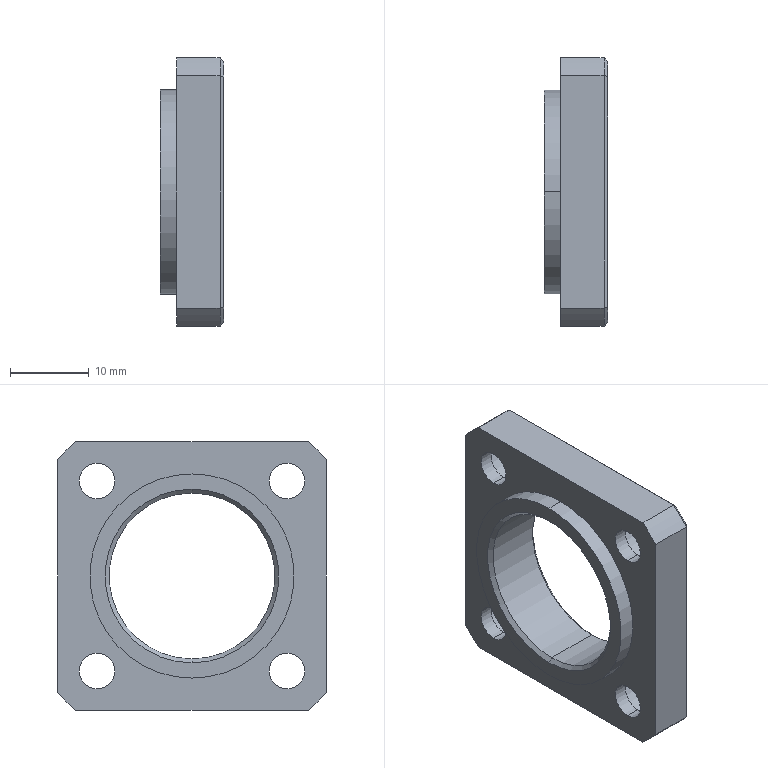Part | SolidWorks | features BaseBody 1 | 1 solid | 47 faces | box 8.1 x 34 x 34 mm | volume 4182 mm3 | cylinder 24 | plane 15 | cone 8 | commonest cylinder face diameters 4.5 x8 8 x8 45 x4 21 x2 25.85 x2
STEP:
#1=CARTESIAN_POINT('',(-6.,0.,12.925));
#2=VERTEX_POINT('',#1);
#3=CARTESIAN_POINT('',(-6.,0.,-12.925));
#4=VERTEX_POINT('',#3);
#5=CARTESIAN_POINT('',(-6.,0.,0.));
#6=DIRECTION('',(-1.,0.,0.));
#7=DIRECTION('',(0.,0.,1.));
#8=AXIS2_PLACEMENT_3D('',#5,#6,#7);
#9=CIRCLE('',#8,12.925);
#10=EDGE_CURVE('',#2,#4,#9,.T.);
#11=ORIENTED_EDGE('',*,*,#10,.T.);
#12=CARTESIAN_POINT('',(-8.1,0.,-12.925));
#13=VERTEX_POINT('',#12);
#14=CARTESIAN_POINT('',(0.,0.,-12.925));
#15=DIRECTION('',(-1.,0.,0.));
#16=VECTOR('',#15,1000.);
#17=LINE('',#14,#16);
#18=EDGE_CURVE('',#4,#13,#17,.T.);
#19=ORIENTED_EDGE('',*,*,#18,.T.);
#20=CARTESIAN_POINT('',(-8.1,0.,12.925));
#21=VERTEX_POINT('',#20);
#22=CARTESIAN_POINT('',(-8.1,0.,0.));
#23=DIRECTION('',(1.,0.,0.));
#24=DIRECTION('',(0.,0.,1.));
#25=AXIS2_PLACEMENT_3D('',#22,#23,#24);
#26=CIRCLE('',#25,12.925);
#27=EDGE_CURVE('',#13,#21,#26,.T.);
#28=ORIENTED_EDGE('',*,*,#27,.T.);
#29=CARTESIAN_POINT('',(0.,0.,12.925));
#30=DIRECTION('',(-1.,0.,0.));
#31=VECTOR('',#30,1000.);
#32=LINE('',#29,#31);
#33=EDGE_CURVE('',#2,#21,#32,.T.);
#34=ORIENTED_EDGE('',*,*,#33,.F.);
#35=EDGE_LOOP('',(#11,#19,#28,#34));
#36=FACE_OUTER_BOUND('',#35,.T.);
#37=CARTESIAN_POINT('',(0.,0.,0.));
#38=DIRECTION('',(-1.,0.,0.));
#39=DIRECTION('',(0.,0.,1.));
#40=AXIS2_PLACEMENT_3D('',#37,#38,#39);
#41=CYLINDRICAL_SURFACE('',#40,12.925);
#42=ADVANCED_FACE('',(#36),#41,.T.);
#43=CARTESIAN_POINT('',(-6.,12.021,-14.271));
#44=VERTEX_POINT('',#43);
#45=CARTESIAN_POINT('',(-6.,12.021,-9.771));
#46=VERTEX_POINT('',#45);
#47=CARTESIAN_POINT('',(-6.,12.021,-12.021));
#48=DIRECTION('',(-1.,0.,0.));
#49=DIRECTION('',(0.,0.,-1.));
#50=AXIS2_PLACEMENT_3D('',#47,#48,#49);
#51=CIRCLE('',#50,2.25);
#52=EDGE_CURVE('',#44,#46,#51,.T.);
#53=ORIENTED_EDGE('',*,*,#52,.T.);
#54=CARTESIAN_POINT('',(-4.2,12.021,-9.771));
#55=VERTEX_POINT('',#54);
#56=CARTESIAN_POINT('',(-8.1,12.021,-9.771));
#57=DIRECTION('',(1.,0.,0.));
#58=VECTOR('',#57,1000.);
#59=LINE('',#56,#58);
#60=EDGE_CURVE('',#46,#55,#59,.T.);
#61=ORIENTED_EDGE('',*,*,#60,.T.);
#62=CARTESIAN_POINT('',(-4.2,12.021,-14.271));
#63=VERTEX_POINT('',#62);
#64=CARTESIAN_POINT('',(-4.2,12.021,-12.021));
#65=DIRECTION('',(-1.,0.,0.));
#66=DIRECTION('',(0.,0.,-1.));
#67=AXIS2_PLACEMENT_3D('',#64,#65,#66);
#68=CIRCLE('',#67,2.25);
#69=EDGE_CURVE('',#63,#55,#68,.T.);
#70=ORIENTED_EDGE('',*,*,#69,.F.);
#71=CARTESIAN_POINT('',(-8.1,12.021,-14.271));
#72=DIRECTION('',(1.,0.,0.));
#73=VECTOR('',#72,1000.);
#74=LINE('',#71,#73);
#75=EDGE_CURVE('',#44,#63,#74,.T.);
#76=ORIENTED_EDGE('',*,*,#75,.F.);
#77=EDGE_LOOP('',(#53,#61,#70,#76));
#78=FACE_OUTER_BOUND('',#77,.T.);
#79=CARTESIAN_POINT('',(-8.1,12.021,-12.021));
#80=DIRECTION('',(1.,0.,0.));
#81=DIRECTION('',(0.,0.,-1.));
#82=AXIS2_PLACEMENT_3D('',#79,#80,#81);
#83=CYLINDRICAL_SURFACE('',#82,2.25);
#84=ADVANCED_FACE('',(#78),#83,.F.);
#85=CARTESIAN_POINT('',(-6.,-12.021,-14.271));
#86=VERTEX_POINT('',#85);
#87=CARTESIAN_POINT('',(-6.,-12.021,-9.771));
#88=VERTEX_POINT('',#87);
#89=CARTESIAN_POINT('',(-6.,-12.021,-12.021));
#90=DIRECTION('',(-1.,0.,0.));
#91=DIRECTION('',(0.,0.,-1.));
#92=AXIS2_PLACEMENT_3D('',#89,#90,#91);
#93=CIRCLE('',#92,2.25);
#94=EDGE_CURVE('',#86,#88,#93,.T.);
#95=ORIENTED_EDGE('',*,*,#94,.T.);
#96=CARTESIAN_POINT('',(-4.2,-12.021,-9.771));
#97=VERTEX_POINT('',#96);
#98=CARTESIAN_POINT('',(-8.1,-12.021,-9.771));
#99=DIRECTION('',(1.,0.,0.));
#100=VECTOR('',#99,1000.);
#101=LINE('',#98,#100);
#102=EDGE_CURVE('',#88,#97,#101,.T.);
#103=ORIENTED_EDGE('',*,*,#102,.T.);
#104=CARTESIAN_POINT('',(-4.2,-12.021,-14.271));
#105=VERTEX_POINT('',#104);
#106=CARTESIAN_POINT('',(-4.2,-12.021,-12.021));
#107=DIRECTION('',(-1.,0.,0.));
#108=DIRECTION('',(0.,0.,-1.));
#109=AXIS2_PLACEMENT_3D('',#106,#107,#108);
#110=CIRCLE('',#109,2.25);
#111=EDGE_CURVE('',#105,#97,#110,.T.);
#112=ORIENTED_EDGE('',*,*,#111,.F.);
#113=CARTESIAN_POINT('',(-8.1,-12.021,-14.271));
#114=DIRECTION('',(1.,0.,0.));
#115=VECTOR('',#114,1000.);
#116=LINE('',#113,#115);
#117=EDGE_CURVE('',#86,#105,#116,.T.);
#118=ORIENTED_EDGE('',*,*,#117,.F.);
#119=EDGE_LOOP('',(#95,#103,#112,#118));
#120=FACE_OUTER_BOUND('',#119,.T.);
#121=CARTESIAN_POINT('',(-8.1,-12.021,-12.021));
#122=DIRECTION('',(1.,0.,0.));
#123=DIRECTION('',(0.,0.,-1.));
#124=AXIS2_PLACEMENT_3D('',#121,#122,#123);
#125=CYLINDRICAL_SURFACE('',#124,2.25);
#126=ADVANCED_FACE('',(#120),#125,.F.);
#127=CARTESIAN_POINT('',(-6.,-12.021,9.771));
#128=VERTEX_POINT('',#127);
#129=CARTESIAN_POINT('',(-6.,-12.021,14.271));
#130=VERTEX_POINT('',#129);
#131=CARTESIAN_POINT('',(-6.,-12.021,12.021));
#132=DIRECTION('',(-1.,0.,0.));
#133=DIRECTION('',(0.,0.,-1.));
#134=AXIS2_PLACEMENT_3D('',#131,#132,#133);
#135=CIRCLE('',#134,2.25);
#136=EDGE_CURVE('',#128,#130,#135,.T.);
#137=ORIENTED_EDGE('',*,*,#136,.T.);
#138=CARTESIAN_POINT('',(-4.2,-12.021,14.271));
#139=VERTEX_POINT('',#138);
#140=CARTESIAN_POINT('',(-8.1,-12.021,14.271));
#141=DIRECTION('',(1.,0.,0.));
#142=VECTOR('',#141,1000.);
#143=LINE('',#140,#142);
#144=EDGE_CURVE('',#130,#139,#143,.T.);
#145=ORIENTED_EDGE('',*,*,#144,.T.);
#146=CARTESIAN_POINT('',(-4.2,-12.021,9.771));
#147=VERTEX_POINT('',#146);
#148=CARTESIAN_POINT('',(-4.2,-12.021,12.021));
#149=DIRECTION('',(-1.,0.,0.));
#150=DIRECTION('',(0.,0.,-1.));
#151=AXIS2_PLACEMENT_3D('',#148,#149,#150);
#152=CIRCLE('',#151,2.25);
#153=EDGE_CURVE('',#147,#139,#152,.T.);
#154=ORIENTED_EDGE('',*,*,#153,.F.);
#155=CARTESIAN_POINT('',(-8.1,-12.021,9.771));
#156=DIRECTION('',(1.,0.,0.));
#157=VECTOR('',#156,1000.);
#158=LINE('',#155,#157);
#159=EDGE_CURVE('',#128,#147,#158,.T.);
#160=ORIENTED_EDGE('',*,*,#159,.F.);
#161=EDGE_LOOP('',(#137,#145,#154,#160));
#162=FACE_OUTER_BOUND('',#161,.T.);
#163=CARTESIAN_POINT('',(-8.1,-12.021,12.021));
#164=DIRECTION('',(1.,0.,0.));
#165=DIRECTION('',(0.,0.,-1.));
#166=AXIS2_PLACEMENT_3D('',#163,#164,#165);
#167=CYLINDRICAL_SURFACE('',#166,2.25);
#168=ADVANCED_FACE('',(#162),#167,.F.);
#169=CARTESIAN_POINT('',(-6.,12.021,9.771));
#170=VERTEX_POINT('',#169);
#171=CARTESIAN_POINT('',(-6.,12.021,14.271));
#172=VERTEX_POINT('',#171);
#173=CARTESIAN_POINT('',(-6.,12.021,12.021));
#174=DIRECTION('',(-1.,0.,0.));
#175=DIRECTION('',(0.,0.,-1.));
#176=AXIS2_PLACEMENT_3D('',#173,#174,#175);
#177=CIRCLE('',#176,2.25);
#178=EDGE_CURVE('',#170,#172,#177,.T.);
#179=ORIENTED_EDGE('',*,*,#178,.T.);
#180=CARTESIAN_POINT('',(-4.2,12.021,14.271));
#181=VERTEX_POINT('',#180);
#182=CARTESIAN_POINT('',(-8.1,12.021,14.271));
#183=DIRECTION('',(1.,0.,0.));
#184=VECTOR('',#183,1000.);
#185=LINE('',#182,#184);
#186=EDGE_CURVE('',#172,#181,#185,.T.);
#187=ORIENTED_EDGE('',*,*,#186,.T.);
#188=CARTESIAN_POINT('',(-4.2,12.021,9.771));
#189=VERTEX_POINT('',#188);
#190=CARTESIAN_POINT('',(-4.2,12.021,12.021));
#191=DIRECTION('',(-1.,0.,0.));
#192=DIRECTION('',(0.,0.,-1.));
#193=AXIS2_PLACEMENT_3D('',#190,#191,#192);
#194=CIRCLE('',#193,2.25);
#195=EDGE_CURVE('',#189,#181,#194,.T.);
#196=ORIENTED_EDGE('',*,*,#195,.F.);
#197=CARTESIAN_POINT('',(-8.1,12.021,9.771));
#198=DIRECTION('',(1.,0.,0.));
#199=VECTOR('',#198,1000.);
#200=LINE('',#197,#199);
#201=EDGE_CURVE('',#170,#189,#200,.T.);
#202=ORIENTED_EDGE('',*,*,#201,.F.);
#203=EDGE_LOOP('',(#179,#187,#196,#202));
#204=FACE_OUTER_BOUND('',#203,.T.);
#205=CARTESIAN_POINT('',(-8.1,12.021,12.021));
#206=DIRECTION('',(1.,0.,0.));
#207=DIRECTION('',(0.,0.,-1.));
#208=AXIS2_PLACEMENT_3D('',#205,#206,#207);
#209=CYLINDRICAL_SURFACE('',#208,2.25);
#210=ADVANCED_FACE('',(#204),#209,.F.);
#211=CARTESIAN_POINT('',(-7.6,0.,-10.5));
#212=VERTEX_POINT('',#211);
#213=CARTESIAN_POINT('',(-7.6,0.,10.5));
#214=VERTEX_POINT('',#213);
#215=CARTESIAN_POINT('',(-7.6,0.,0.));
#216=DIRECTION('',(-1.,0.,0.));
#217=DIRECTION('',(0.,0.,1.));
#218=AXIS2_PLACEMENT_3D('',#215,#216,#217);
#219=CIRCLE('',#218,10.5);
#220=EDGE_CURVE('',#212,#214,#219,.T.);
#221=ORIENTED_EDGE('',*,*,#220,.F.);
#222=CARTESIAN_POINT('',(-8.1,0.,-11.));
#223=VERTEX_POINT('',#222);
#224=CARTESIAN_POINT('',(-8.1,0.,-11.));
#225=DIRECTION('',(-0.7071,0.,-0.7071));
#226=VECTOR('',#225,1000.);
#227=LINE('',#224,#226);
#228=EDGE_CURVE('',#212,#223,#227,.T.);
#229=ORIENTED_EDGE('',*,*,#228,.T.);
#230=CARTESIAN_POINT('',(-8.1,0.,11.));
#231=VERTEX_POINT('',#230);
#232=CARTESIAN_POINT('',(-8.1,0.,0.));
#233=DIRECTION('',(-1.,0.,0.));
#234=DIRECTION('',(0.,0.,1.));
#235=AXIS2_PLACEMENT_3D('',#232,#233,#234);
#236=CIRCLE('',#235,11.);
#237=EDGE_CURVE('',#223,#231,#236,.T.);
#238=ORIENTED_EDGE('',*,*,#237,.T.);
#239=CARTESIAN_POINT('',(-8.1,0.,11.));
#240=DIRECTION('',(-0.7071,0.,0.7071));
#241=VECTOR('',#240,1000.);
#242=LINE('',#239,#241);
#243=EDGE_CURVE('',#214,#231,#242,.T.);
#244=ORIENTED_EDGE('',*,*,#243,.F.);
#245=EDGE_LOOP('',(#221,#229,#238,#244));
#246=FACE_OUTER_BOUND('',#245,.T.);
#247=CARTESIAN_POINT('',(-8.1,0.,0.));
#248=DIRECTION('',(-1.,0.,0.));
#249=DIRECTION('',(0.,0.,1.));
#250=AXIS2_PLACEMENT_3D('',#247,#248,#249);
#251=CONICAL_SURFACE('',#250,11.,0.7854);
#252=ADVANCED_FACE('',(#246),#251,.F.);
#253=CARTESIAN_POINT('',(-4.2,12.021,-8.021));
#254=VERTEX_POINT('',#253);
#255=CARTESIAN_POINT('',(-4.2,12.021,-16.021));
#256=VERTEX_POINT('',#255);
#257=CARTESIAN_POINT('',(-4.2,12.021,-12.021));
#258=DIRECTION('',(1.,0.,0.));
#259=DIRECTION('',(0.,0.,-1.));
#260=AXIS2_PLACEMENT_3D('',#257,#258,#259);
#261=CIRCLE('',#260,4.);
#262=EDGE_CURVE('',#254,#256,#261,.T.);
#263=ORIENTED_EDGE('',*,*,#262,.F.);
#264=CARTESIAN_POINT('',(0.,12.021,-8.021));
#265=VERTEX_POINT('',#264);
#266=CARTESIAN_POINT('',(-8.1,12.021,-8.021));
#267=DIRECTION('',(1.,0.,0.));
#268=VECTOR('',#267,1000.);
#269=LINE('',#266,#268);
#270=EDGE_CURVE('',#254,#265,#269,.T.);
#271=ORIENTED_EDGE('',*,*,#270,.T.);
#272=CARTESIAN_POINT('',(0.,12.021,-16.021));
#273=VERTEX_POINT('',#272);
#274=CARTESIAN_POINT('',(0.,12.021,-12.021));
#275=DIRECTION('',(-1.,0.,0.));
#276=DIRECTION('',(0.,0.,-1.));
#277=AXIS2_PLACEMENT_3D('',#274,#275,#276);
#278=CIRCLE('',#277,4.);
#279=EDGE_CURVE('',#273,#265,#278,.T.);
#280=ORIENTED_EDGE('',*,*,#279,.F.);
#281=CARTESIAN_POINT('',(-8.1,12.021,-16.021));
#282=DIRECTION('',(1.,0.,0.));
#283=VECTOR('',#282,1000.);
#284=LINE('',#281,#283);
#285=EDGE_CURVE('',#256,#273,#284,.T.);
#286=ORIENTED_EDGE('',*,*,#285,.F.);
#287=EDGE_LOOP('',(#263,#271,#280,#286));
#288=FACE_OUTER_BOUND('',#287,.T.);
#289=CARTESIAN_POINT('',(-8.1,12.021,-12.021));
#290=DIRECTION('',(1.,0.,0.));
#291=DIRECTION('',(0.,0.,-1.));
#292=AXIS2_PLACEMENT_3D('',#289,#290,#291);
#293=CYLINDRICAL_SURFACE('',#292,4.);
#294=ADVANCED_FACE('',(#288),#293,.F.);
#295=CARTESIAN_POINT('',(-4.2,-12.021,-8.021));
#296=VERTEX_POINT('',#295);
#297=CARTESIAN_POINT('',(-4.2,-12.021,-16.021));
#298=VERTEX_POINT('',#297);
#299=CARTESIAN_POINT('',(-4.2,-12.021,-12.021));
#300=DIRECTION('',(1.,0.,0.));
#301=DIRECTION('',(0.,0.,-1.));
#302=AXIS2_PLACEMENT_3D('',#299,#300,#301);
#303=CIRCLE('',#302,4.);
#304=EDGE_CURVE('',#296,#298,#303,.T.);
#305=ORIENTED_EDGE('',*,*,#304,.F.);
#306=CARTESIAN_POINT('',(0.,-12.021,-8.021));
#307=VERTEX_POINT('',#306);
#308=CARTESIAN_POINT('',(-8.1,-12.021,-8.021));
#309=DIRECTION('',(1.,0.,0.));
#310=VECTOR('',#309,1000.);
#311=LINE('',#308,#310);
#312=EDGE_CURVE('',#296,#307,#311,.T.);
#313=ORIENTED_EDGE('',*,*,#312,.T.);
#314=CARTESIAN_POINT('',(0.,-12.021,-16.021));
#315=VERTEX_POINT('',#314);
#316=CARTESIAN_POINT('',(0.,-12.021,-12.021));
#317=DIRECTION('',(-1.,0.,0.));
#318=DIRECTION('',(0.,0.,-1.));
#319=AXIS2_PLACEMENT_3D('',#316,#317,#318);
#320=CIRCLE('',#319,4.);
#321=EDGE_CURVE('',#315,#307,#320,.T.);
#322=ORIENTED_EDGE('',*,*,#321,.F.);
#323=CARTESIAN_POINT('',(-8.1,-12.021,-16.021));
#324=DIRECTION('',(1.,0.,0.));
#325=VECTOR('',#324,1000.);
#326=LINE('',#323,#325);
#327=EDGE_CURVE('',#298,#315,#326,.T.);
#328=ORIENTED_EDGE('',*,*,#327,.F.);
#329=EDGE_LOOP('',(#305,#313,#322,#328));
#330=FACE_OUTER_BOUND('',#329,.T.);
#331=CARTESIAN_POINT('',(-8.1,-12.021,-12.021));
#332=DIRECTION('',(1.,0.,0.));
#333=DIRECTION('',(0.,0.,-1.));
#334=AXIS2_PLACEMENT_3D('',#331,#332,#333);
#335=CYLINDRICAL_SURFACE('',#334,4.);
#336=ADVANCED_FACE('',(#330),#335,.F.);
#337=CARTESIAN_POINT('',(-4.2,-12.021,16.021));
#338=VERTEX_POINT('',#337);
#339=CARTESIAN_POINT('',(-4.2,-12.021,8.021));
#340=VERTEX_POINT('',#339);
#341=CARTESIAN_POINT('',(-4.2,-12.021,12.021));
#342=DIRECTION('',(1.,0.,0.));
#343=DIRECTION('',(0.,0.,-1.));
#344=AXIS2_PLACEMENT_3D('',#341,#342,#343);
#345=CIRCLE('',#344,4.);
#346=EDGE_CURVE('',#338,#340,#345,.T.);
#347=ORIENTED_EDGE('',*,*,#346,.F.);
#348=CARTESIAN_POINT('',(0.,-12.021,16.021));
#349=VERTEX_POINT('',#348);
#350=CARTESIAN_POINT('',(-8.1,-12.021,16.021));
#351=DIRECTION('',(1.,0.,0.));
#352=VECTOR('',#351,1000.);
#353=LINE('',#350,#352);
#354=EDGE_CURVE('',#338,#349,#353,.T.);
#355=ORIENTED_EDGE('',*,*,#354,.T.);
#356=CARTESIAN_POINT('',(0.,-12.021,8.021));
#357=VERTEX_POINT('',#356);
#358=CARTESIAN_POINT('',(0.,-12.021,12.021));
#359=DIRECTION('',(-1.,0.,0.));
#360=DIRECTION('',(0.,0.,-1.));
#361=AXIS2_PLACEMENT_3D('',#358,#359,#360);
#362=CIRCLE('',#361,4.);
#363=EDGE_CURVE('',#357,#349,#362,.T.);
#364=ORIENTED_EDGE('',*,*,#363,.F.);
#365=CARTESIAN_POINT('',(-8.1,-12.021,8.021));
#366=DIRECTION('',(1.,0.,0.));
#367=VECTOR('',#366,1000.);
#368=LINE('',#365,#367);
#369=EDGE_CURVE('',#340,#357,#368,.T.);
#370=ORIENTED_EDGE('',*,*,#369,.F.);
#371=EDGE_LOOP('',(#347,#355,#364,#370));
#372=FACE_OUTER_BOUND('',#371,.T.);
#373=CARTESIAN_POINT('',(-8.1,-12.021,12.021));
#374=DIRECTION('',(1.,0.,0.));
#375=DIRECTION('',(0.,0.,-1.));
#376=AXIS2_PLACEMENT_3D('',#373,#374,#375);
#377=CYLINDRICAL_SURFACE('',#376,4.);
#378=ADVANCED_FACE('',(#372),#377,.F.);
#379=CARTESIAN_POINT('',(-4.2,12.021,16.021));
#380=VERTEX_POINT('',#379);
#381=CARTESIAN_POINT('',(-4.2,12.021,8.021));
#382=VERTEX_POINT('',#381);
#383=CARTESIAN_POINT('',(-4.2,12.021,12.021));
#384=DIRECTION('',(1.,0.,0.));
#385=DIRECTION('',(0.,0.,-1.));
#386=AXIS2_PLACEMENT_3D('',#383,#384,#385);
#387=CIRCLE('',#386,4.);
#388=EDGE_CURVE('',#380,#382,#387,.T.);
#389=ORIENTED_EDGE('',*,*,#388,.F.);
#390=CARTESIAN_POINT('',(0.,12.021,16.021));
#391=VERTEX_POINT('',#390);
#392=CARTESIAN_POINT('',(-8.1,12.021,16.021));
#393=DIRECTION('',(1.,0.,0.));
#394=VECTOR('',#393,1000.);
#395=LINE('',#392,#394);
#396=EDGE_CURVE('',#380,#391,#395,.T.);
#397=ORIENTED_EDGE('',*,*,#396,.T.);
#398=CARTESIAN_POINT('',(0.,12.021,8.021));
#399=VERTEX_POINT('',#398);
#400=CARTESIAN_POINT('',(0.,12.021,12.021));
#401=DIRECTION('',(-1.,0.,0.));
#402=DIRECTION('',(0.,0.,-1.));
#403=AXIS2_PLACEMENT_3D('',#400,#401,#402);
#404=CIRCLE('',#403,4.);
#405=EDGE_CURVE('',#399,#391,#404,.T.);
#406=ORIENTED_EDGE('',*,*,#405,.F.);
#407=CARTESIAN_POINT('',(-8.1,12.021,8.021));
#408=DIRECTION('',(1.,0.,0.));
#409=VECTOR('',#408,1000.);
#410=LINE('',#407,#409);
#411=EDGE_CURVE('',#382,#399,#410,.T.);
#412=ORIENTED_EDGE('',*,*,#411,.F.);
#413=EDGE_LOOP('',(#389,#397,#406,#412));
#414=FACE_OUTER_BOUND('',#413,.T.);
#415=CARTESIAN_POINT('',(-8.1,12.021,12.021));
#416=DIRECTION('',(1.,0.,0.));
#417=DIRECTION('',(0.,0.,-1.));
#418=AXIS2_PLACEMENT_3D('',#415,#416,#417);
#419=CYLINDRICAL_SURFACE('',#418,4.);
#420=ADVANCED_FACE('',(#414),#419,.F.);
#421=CARTESIAN_POINT('',(-0.5,0.,-10.5));
#422=VERTEX_POINT('',#421);
#423=CARTESIAN_POINT('',(-0.5,0.,10.5));
#424=VERTEX_POINT('',#423);
#425=CARTESIAN_POINT('',(-0.5,0.,0.));
#426=DIRECTION('',(-1.,0.,0.));
#427=DIRECTION('',(0.,0.,1.));
#428=AXIS2_PLACEMENT_3D('',#425,#426,#427);
#429=CIRCLE('',#428,10.5);
#430=EDGE_CURVE('',#422,#424,#429,.T.);
#431=ORIENTED_EDGE('',*,*,#430,.F.);
#432=CARTESIAN_POINT('',(0.,0.,-10.5));
#433=DIRECTION('',(-1.,0.,0.));
#434=VECTOR('',#433,1000.);
#435=LINE('',#432,#434);
#436=EDGE_CURVE('',#422,#212,#435,.T.);
#437=ORIENTED_EDGE('',*,*,#436,.T.);
#438=ORIENTED_EDGE('',*,*,#220,.T.);
#439=CARTESIAN_POINT('',(0.,0.,10.5));
#440=DIRECTION('',(-1.,0.,0.));
#441=VECTOR('',#440,1000.);
#442=LINE('',#439,#441);
#443=EDGE_CURVE('',#424,#214,#442,.T.);
#444=ORIENTED_EDGE('',*,*,#443,.F.);
#445=EDGE_LOOP('',(#431,#437,#438,#444));
#446=FACE_OUTER_BOUND('',#445,.T.);
#447=CARTESIAN_POINT('',(0.,0.,0.));
#448=DIRECTION('',(-1.,0.,0.));
#449=DIRECTION('',(0.,0.,1.));
#450=AXIS2_PLACEMENT_3D('',#447,#448,#449);
#451=CYLINDRICAL_SURFACE('',#450,10.5);
#452=ADVANCED_FACE('',(#446),#451,.F.);
#453=ORIENTED_EDGE('',*,*,#430,.T.);
#454=CARTESIAN_POINT('',(0.,0.,11.));
#455=VERTEX_POINT('',#454);
#456=CARTESIAN_POINT('',(0.,0.,11.));
#457=DIRECTION('',(0.7071,0.,0.7071));
#458=VECTOR('',#457,1000.);
#459=LINE('',#456,#458);
#460=EDGE_CURVE('',#424,#455,#459,.T.);
#461=ORIENTED_EDGE('',*,*,#460,.T.);
#462=CARTESIAN_POINT('',(0.,0.,-11.));
#463=VERTEX_POINT('',#462);
#464=CARTESIAN_POINT('',(0.,0.,0.));
#465=DIRECTION('',(1.,0.,0.));
#466=DIRECTION('',(0.,0.,-1.));
#467=AXIS2_PLACEMENT_3D('',#464,#465,#466);
#468=CIRCLE('',#467,11.);
#469=EDGE_CURVE('',#455,#463,#468,.T.);
#470=ORIENTED_EDGE('',*,*,#469,.T.);
#471=CARTESIAN_POINT('',(0.,0.,-11.));
#472=DIRECTION('',(0.7071,0.,-0.7071));
#473=VECTOR('',#472,1000.);
#474=LINE('',#471,#473);
#475=EDGE_CURVE('',#422,#463,#474,.T.);
#476=ORIENTED_EDGE('',*,*,#475,.F.);
#477=EDGE_LOOP('',(#453,#461,#470,#476));
#478=FACE_OUTER_BOUND('',#477,.T.);
#479=CARTESIAN_POINT('',(0.,0.,0.));
#480=DIRECTION('',(1.,0.,0.));
#481=DIRECTION('',(0.,0.,-1.));
#482=AXIS2_PLACEMENT_3D('',#479,#480,#481);
#483=CONICAL_SURFACE('',#482,11.,0.7854);
#484=ADVANCED_FACE('',(#478),#483,.F.);
#485=ORIENTED_EDGE('',*,*,#10,.F.);
#486=CARTESIAN_POINT('',(-6.,0.,0.));
#487=DIRECTION('',(-1.,0.,0.));
#488=DIRECTION('',(0.,0.,1.));
#489=AXIS2_PLACEMENT_3D('',#486,#487,#488);
#490=CIRCLE('',#489,12.925);
#491=EDGE_CURVE('',#4,#2,#490,.T.);
#492=ORIENTED_EDGE('',*,*,#491,.F.);
#493=EDGE_LOOP('',(#485,#492));
#494=FACE_BOUND('',#493,.T.);
#495=ORIENTED_EDGE('',*,*,#52,.F.);
#496=CARTESIAN_POINT('',(-6.,12.021,-12.021));
#497=DIRECTION('',(-1.,0.,0.));
#498=DIRECTION('',(0.,0.,-1.));
#499=AXIS2_PLACEMENT_3D('',#496,#497,#498);
#500=CIRCLE('',#499,2.25);
#501=EDGE_CURVE('',#46,#44,#500,.T.);
#502=ORIENTED_EDGE('',*,*,#501,.F.);
#503=EDGE_LOOP('',(#495,#502));
#504=FACE_BOUND('',#503,.T.);
#505=ORIENTED_EDGE('',*,*,#94,.F.);
#506=CARTESIAN_POINT('',(-6.,-12.021,-12.021));
#507=DIRECTION('',(-1.,0.,0.));
#508=DIRECTION('',(0.,0.,-1.));
#509=AXIS2_PLACEMENT_3D('',#506,#507,#508);
#510=CIRCLE('',#509,2.25);
#511=EDGE_CURVE('',#88,#86,#510,.T.);
#512=ORIENTED_EDGE('',*,*,#511,.F.);
#513=EDGE_LOOP('',(#505,#512));
#514=FACE_BOUND('',#513,.T.);
#515=ORIENTED_EDGE('',*,*,#136,.F.);
#516=CARTESIAN_POINT('',(-6.,-12.021,12.021));
#517=DIRECTION('',(-1.,0.,0.));
#518=DIRECTION('',(0.,0.,-1.));
#519=AXIS2_PLACEMENT_3D('',#516,#517,#518);
#520=CIRCLE('',#519,2.25);
#521=EDGE_CURVE('',#130,#128,#520,.T.);
#522=ORIENTED_EDGE('',*,*,#521,.F.);
#523=EDGE_LOOP('',(#515,#522));
#524=FACE_BOUND('',#523,.T.);
#525=ORIENTED_EDGE('',*,*,#178,.F.);
#526=CARTESIAN_POINT('',(-6.,12.021,12.021));
#527=DIRECTION('',(-1.,0.,0.));
#528=DIRECTION('',(0.,0.,-1.));
#529=AXIS2_PLACEMENT_3D('',#526,#527,#528);
#530=CIRCLE('',#529,2.25);
#531=EDGE_CURVE('',#172,#170,#530,.T.);
#532=ORIENTED_EDGE('',*,*,#531,.F.);
#533=EDGE_LOOP('',(#525,#532));
#534=FACE_BOUND('',#533,.T.);
#535=CARTESIAN_POINT('',(-6.,14.739,-17.));
#536=VERTEX_POINT('',#535);
#537=CARTESIAN_POINT('',(-6.,17.,-14.739));
#538=VERTEX_POINT('',#537);
#539=CARTESIAN_POINT('',(-6.,0.,0.));
#540=DIRECTION('',(1.,0.,0.));
#541=DIRECTION('',(0.,0.,1.));
#542=AXIS2_PLACEMENT_3D('',#539,#540,#541);
#543=CIRCLE('',#542,22.5);
#544=EDGE_CURVE('',#536,#538,#543,.T.);
#545=ORIENTED_EDGE('',*,*,#544,.F.);
#546=CARTESIAN_POINT('',(-6.,-14.739,-17.));
#547=VERTEX_POINT('',#546);
#548=CARTESIAN_POINT('',(-6.,12.925,-17.));
#549=DIRECTION('',(0.,1.,0.));
#550=VECTOR('',#549,1000.);
#551=LINE('',#548,#550);
#552=EDGE_CURVE('',#547,#536,#551,.T.);
#553=ORIENTED_EDGE('',*,*,#552,.F.);
#554=CARTESIAN_POINT('',(-6.,-17.,-14.739));
#555=VERTEX_POINT('',#554);
#556=CARTESIAN_POINT('',(-6.,0.,0.));
#557=DIRECTION('',(1.,0.,0.));
#558=DIRECTION('',(0.,0.,1.));
#559=AXIS2_PLACEMENT_3D('',#556,#557,#558);
#560=CIRCLE('',#559,22.5);
#561=EDGE_CURVE('',#555,#547,#560,.T.);
#562=ORIENTED_EDGE('',*,*,#561,.F.);
#563=CARTESIAN_POINT('',(-6.,-17.,14.739));
#564=VERTEX_POINT('',#563);
#565=CARTESIAN_POINT('',(-6.,-17.,0.));
#566=DIRECTION('',(0.,0.,-1.));
#567=VECTOR('',#566,1000.);
#568=LINE('',#565,#567);
#569=EDGE_CURVE('',#564,#555,#568,.T.);
#570=ORIENTED_EDGE('',*,*,#569,.F.);
#571=CARTESIAN_POINT('',(-6.,-14.739,17.));
#572=VERTEX_POINT('',#571);
#573=CARTESIAN_POINT('',(-6.,0.,0.));
#574=DIRECTION('',(1.,0.,0.));
#575=DIRECTION('',(0.,0.,1.));
#576=AXIS2_PLACEMENT_3D('',#573,#574,#575);
#577=CIRCLE('',#576,22.5);
#578=EDGE_CURVE('',#572,#564,#577,.T.);
#579=ORIENTED_EDGE('',*,*,#578,.F.);
#580=CARTESIAN_POINT('',(-6.,14.739,17.));
#581=VERTEX_POINT('',#580);
#582=CARTESIAN_POINT('',(-6.,12.925,17.));
#583=DIRECTION('',(0.,-1.,0.));
#584=VECTOR('',#583,1000.);
#585=LINE('',#582,#584);
#586=EDGE_CURVE('',#581,#572,#585,.T.);
#587=ORIENTED_EDGE('',*,*,#586,.F.);
#588=CARTESIAN_POINT('',(-6.,17.,14.739));
#589=VERTEX_POINT('',#588);
#590=CARTESIAN_POINT('',(-6.,0.,0.));
#591=DIRECTION('',(1.,0.,0.));
#592=DIRECTION('',(0.,0.,1.));
#593=AXIS2_PLACEMENT_3D('',#590,#591,#592);
#594=CIRCLE('',#593,22.5);
#595=EDGE_CURVE('',#589,#581,#594,.T.);
#596=ORIENTED_EDGE('',*,*,#595,.F.);
#597=CARTESIAN_POINT('',(-6.,17.,0.));
#598=DIRECTION('',(0.,0.,1.));
#599=VECTOR('',#598,1000.);
#600=LINE('',#597,#599);
#601=EDGE_CURVE('',#538,#589,#600,.T.);
#602=ORIENTED_EDGE('',*,*,#601,.F.);
#603=EDGE_LOOP('',(#545,#553,#562,#570,#579,#587,#596,#602));
#604=FACE_OUTER_BOUND('',#603,.T.);
#605=CARTESIAN_POINT('',(-6.,12.925,0.));
#606=DIRECTION('',(1.,0.,0.));
#607=DIRECTION('',(0.,0.,-1.));
#608=AXIS2_PLACEMENT_3D('',#605,#606,#607);
#609=PLANE('',#608);
#610=ADVANCED_FACE('',(#494,#504,#514,#524,#534,#604),#609,.F.);
#611=ORIENTED_EDGE('',*,*,#18,.F.);
#612=ORIENTED_EDGE('',*,*,#491,.T.);
#613=ORIENTED_EDGE('',*,*,#33,.T.);
#614=CARTESIAN_POINT('',(-8.1,0.,0.));
#615=DIRECTION('',(1.,0.,0.));
#616=DIRECTION('',(0.,0.,1.));
#617=AXIS2_PLACEMENT_3D('',#614,#615,#616);
#618=CIRCLE('',#617,12.925);
#619=EDGE_CURVE('',#21,#13,#618,.T.);
#620=ORIENTED_EDGE('',*,*,#619,.T.);
#621=EDGE_LOOP('',(#611,#612,#613,#620));
#622=FACE_OUTER_BOUND('',#621,.T.);
#623=CARTESIAN_POINT('',(0.,0.,0.));
#624=DIRECTION('',(-1.,0.,0.));
#625=DIRECTION('',(0.,0.,1.));
#626=AXIS2_PLACEMENT_3D('',#623,#624,#625);
#627=CYLINDRICAL_SURFACE('',#626,12.925);
#628=ADVANCED_FACE('',(#622),#627,.T.);
#629=ORIENTED_EDGE('',*,*,#60,.F.);
#630=ORIENTED_EDGE('',*,*,#501,.T.);
#631=ORIENTED_EDGE('',*,*,#75,.T.);
#632=CARTESIAN_POINT('',(-4.2,12.021,-12.021));
#633=DIRECTION('',(-1.,0.,0.));
#634=DIRECTION('',(0.,0.,-1.));
#635=AXIS2_PLACEMENT_3D('',#632,#633,#634);
#636=CIRCLE('',#635,2.25);
#637=EDGE_CURVE('',#55,#63,#636,.T.);
#638=ORIENTED_EDGE('',*,*,#637,.F.);
#639=EDGE_LOOP('',(#629,#630,#631,#638));
#640=FACE_OUTER_BOUND('',#639,.T.);
#641=CARTESIAN_POINT('',(-8.1,12.021,-12.021));
#642=DIRECTION('',(1.,0.,0.));
#643=DIRECTION('',(0.,0.,-1.));
#644=AXIS2_PLACEMENT_3D('',#641,#642,#643);
#645=CYLINDRICAL_SURFACE('',#644,2.25);
#646=ADVANCED_FACE('',(#640),#645,.F.);
#647=ORIENTED_EDGE('',*,*,#102,.F.);
#648=ORIENTED_EDGE('',*,*,#511,.T.);
#649=ORIENTED_EDGE('',*,*,#117,.T.);
#650=CARTESIAN_POINT('',(-4.2,-12.021,-12.021));
#651=DIRECTION('',(-1.,0.,0.));
#652=DIRECTION('',(0.,0.,-1.));
#653=AXIS2_PLACEMENT_3D('',#650,#651,#652);
#654=CIRCLE('',#653,2.25);
#655=EDGE_CURVE('',#97,#105,#654,.T.);
#656=ORIENTED_EDGE('',*,*,#655,.F.);
#657=EDGE_LOOP('',(#647,#648,#649,#656));
#658=FACE_OUTER_BOUND('',#657,.T.);
#659=CARTESIAN_POINT('',(-8.1,-12.021,-12.021));
#660=DIRECTION('',(1.,0.,0.));
#661=DIRECTION('',(0.,0.,-1.));
#662=AXIS2_PLACEMENT_3D('',#659,#660,#661);
#663=CYLINDRICAL_SURFACE('',#662,2.25);
#664=ADVANCED_FACE('',(#658),#663,.F.);
#665=ORIENTED_EDGE('',*,*,#144,.F.);
#666=ORIENTED_EDGE('',*,*,#521,.T.);
#667=ORIENTED_EDGE('',*,*,#159,.T.);
#668=CARTESIAN_POINT('',(-4.2,-12.021,12.021));
#669=DIRECTION('',(-1.,0.,0.));
#670=DIRECTION('',(0.,0.,-1.));
#671=AXIS2_PLACEMENT_3D('',#668,#669,#670);
#672=CIRCLE('',#671,2.25);
#673=EDGE_CURVE('',#139,#147,#672,.T.);
#674=ORIENTED_EDGE('',*,*,#673,.F.);
#675=EDGE_LOOP('',(#665,#666,#667,#674));
#676=FACE_OUTER_BOUND('',#675,.T.);
#677=CARTESIAN_POINT('',(-8.1,-12.021,12.021));
#678=DIRECTION('',(1.,0.,0.));
#679=DIRECTION('',(0.,0.,-1.));
#680=AXIS2_PLACEMENT_3D('',#677,#678,#679);
#681=CYLINDRICAL_SURFACE('',#680,2.25);
#682=ADVANCED_FACE('',(#676),#681,.F.);
#683=ORIENTED_EDGE('',*,*,#186,.F.);
#684=ORIENTED_EDGE('',*,*,#531,.T.);
#685=ORIENTED_EDGE('',*,*,#201,.T.);
#686=CARTESIAN_POINT('',(-4.2,12.021,12.021));
#687=DIRECTION('',(-1.,0.,0.));
#688=DIRECTION('',(0.,0.,-1.));
#689=AXIS2_PLACEMENT_3D('',#686,#687,#688);
#690=CIRCLE('',#689,2.25);
#691=EDGE_CURVE('',#181,#189,#690,.T.);
#692=ORIENTED_EDGE('',*,*,#691,.F.);
#693=EDGE_LOOP('',(#683,#684,#685,#692));
#694=FACE_OUTER_BOUND('',#693,.T.);
#695=CARTESIAN_POINT('',(-8.1,12.021,12.021));
#696=DIRECTION('',(1.,0.,0.));
#697=DIRECTION('',(0.,0.,-1.));
#698=AXIS2_PLACEMENT_3D('',#695,#696,#697);
#699=CYLINDRICAL_SURFACE('',#698,2.25);
#700=ADVANCED_FACE('',(#694),#699,.F.);
#701=CARTESIAN_POINT('',(-0.5,17.,14.739));
#702=VERTEX_POINT('',#701);
#703=CARTESIAN_POINT('',(-0.5,17.,-14.739));
#704=VERTEX_POINT('',#703);
#705=CARTESIAN_POINT('',(-0.5,17.,-17.));
#706=DIRECTION('',(0.,0.,-1.));
#707=VECTOR('',#706,1000.);
#708=LINE('',#705,#707);
#709=EDGE_CURVE('',#702,#704,#708,.T.);
#710=ORIENTED_EDGE('',*,*,#709,.T.);
#711=CARTESIAN_POINT('',(-8.1,17.,-14.739));
#712=DIRECTION('',(-1.,0.,0.));
#713=VECTOR('',#712,1000.);
#714=LINE('',#711,#713);
#715=EDGE_CURVE('',#704,#538,#714,.T.);
#716=ORIENTED_EDGE('',*,*,#715,.T.);
#717=ORIENTED_EDGE('',*,*,#601,.T.);
#718=CARTESIAN_POINT('',(-8.1,17.,14.739));
#719=DIRECTION('',(1.,0.,0.));
#720=VECTOR('',#719,1000.);
#721=LINE('',#718,#720);
#722=EDGE_CURVE('',#589,#702,#721,.T.);
#723=ORIENTED_EDGE('',*,*,#722,.T.);
#724=EDGE_LOOP('',(#710,#716,#717,#723));
#725=FACE_OUTER_BOUND('',#724,.T.);
#726=CARTESIAN_POINT('',(-8.1,17.,-17.));
#727=DIRECTION('',(0.,1.,0.));
#728=DIRECTION('',(0.,0.,1.));
#729=AXIS2_PLACEMENT_3D('',#726,#727,#728);
#730=PLANE('',#729);
#731=ADVANCED_FACE('',(#725),#730,.T.);
#732=ORIENTED_EDGE('',*,*,#715,.F.);
#733=CARTESIAN_POINT('',(-0.5,14.739,-17.));
#734=VERTEX_POINT('',#733);
#735=CARTESIAN_POINT('',(-0.5,0.,0.));
#736=DIRECTION('',(-1.,0.,0.));
#737=DIRECTION('',(0.,0.,1.));
#738=AXIS2_PLACEMENT_3D('',#735,#736,#737);
#739=CIRCLE('',#738,22.5);
#740=EDGE_CURVE('',#704,#734,#739,.T.);
#741=ORIENTED_EDGE('',*,*,#740,.T.);
#742=CARTESIAN_POINT('',(0.,14.739,-17.));
#743=DIRECTION('',(-1.,0.,0.));
#744=VECTOR('',#743,1000.);
#745=LINE('',#742,#744);
#746=EDGE_CURVE('',#734,#536,#745,.T.);
#747=ORIENTED_EDGE('',*,*,#746,.T.);
#748=ORIENTED_EDGE('',*,*,#544,.T.);
#749=EDGE_LOOP('',(#732,#741,#747,#748));
#750=FACE_OUTER_BOUND('',#749,.T.);
#751=CARTESIAN_POINT('',(0.,0.,0.));
#752=DIRECTION('',(-1.,0.,0.));
#753=DIRECTION('',(0.,0.,1.));
#754=AXIS2_PLACEMENT_3D('',#751,#752,#753);
#755=CYLINDRICAL_SURFACE('',#754,22.5);
#756=ADVANCED_FACE('',(#750),#755,.T.);
#757=CARTESIAN_POINT('',(-0.5,-14.739,-17.));
#758=VERTEX_POINT('',#757);
#759=CARTESIAN_POINT('',(-0.5,-17.,-17.));
#760=DIRECTION('',(0.,-1.,0.));
#761=VECTOR('',#760,1000.);
#762=LINE('',#759,#761);
#763=EDGE_CURVE('',#734,#758,#762,.T.);
#764=ORIENTED_EDGE('',*,*,#763,.T.);
#765=CARTESIAN_POINT('',(-8.1,-14.739,-17.));
#766=DIRECTION('',(-1.,0.,0.));
#767=VECTOR('',#766,1000.);
#768=LINE('',#765,#767);
#769=EDGE_CURVE('',#758,#547,#768,.T.);
#770=ORIENTED_EDGE('',*,*,#769,.T.);
#771=ORIENTED_EDGE('',*,*,#552,.T.);
#772=ORIENTED_EDGE('',*,*,#746,.F.);
#773=EDGE_LOOP('',(#764,#770,#771,#772));
#774=FACE_OUTER_BOUND('',#773,.T.);
#775=CARTESIAN_POINT('',(-8.1,-17.,-17.));
#776=DIRECTION('',(0.,0.,-1.));
#777=DIRECTION('',(-1.,0.,0.));
#778=AXIS2_PLACEMENT_3D('',#775,#776,#777);
#779=PLANE('',#778);
#780=ADVANCED_FACE('',(#774),#779,.T.);
#781=ORIENTED_EDGE('',*,*,#769,.F.);
#782=CARTESIAN_POINT('',(-0.5,-17.,-14.739));
#783=VERTEX_POINT('',#782);
#784=CARTESIAN_POINT('',(-0.5,0.,0.));
#785=DIRECTION('',(-1.,0.,0.));
#786=DIRECTION('',(0.,0.,1.));
#787=AXIS2_PLACEMENT_3D('',#784,#785,#786);
#788=CIRCLE('',#787,22.5);
#789=EDGE_CURVE('',#758,#783,#788,.T.);
#790=ORIENTED_EDGE('',*,*,#789,.T.);
#791=CARTESIAN_POINT('',(0.,-17.,-14.739));
#792=DIRECTION('',(-1.,0.,0.));
#793=VECTOR('',#792,1000.);
#794=LINE('',#791,#793);
#795=EDGE_CURVE('',#783,#555,#794,.T.);
#796=ORIENTED_EDGE('',*,*,#795,.T.);
#797=ORIENTED_EDGE('',*,*,#561,.T.);
#798=EDGE_LOOP('',(#781,#790,#796,#797));
#799=FACE_OUTER_BOUND('',#798,.T.);
#800=CARTESIAN_POINT('',(0.,0.,0.));
#801=DIRECTION('',(-1.,0.,0.));
#802=DIRECTION('',(0.,0.,1.));
#803=AXIS2_PLACEMENT_3D('',#800,#801,#802);
#804=CYLINDRICAL_SURFACE('',#803,22.5);
#805=ADVANCED_FACE('',(#799),#804,.T.);
#806=CARTESIAN_POINT('',(-0.5,-17.,14.739));
#807=VERTEX_POINT('',#806);
#808=CARTESIAN_POINT('',(-0.5,-17.,17.));
#809=DIRECTION('',(0.,0.,1.));
#810=VECTOR('',#809,1000.);
#811=LINE('',#808,#810);
#812=EDGE_CURVE('',#783,#807,#811,.T.);
#813=ORIENTED_EDGE('',*,*,#812,.T.);
#814=CARTESIAN_POINT('',(-8.1,-17.,14.739));
#815=DIRECTION('',(-1.,0.,0.));
#816=VECTOR('',#815,1000.);
#817=LINE('',#814,#816);
#818=EDGE_CURVE('',#807,#564,#817,.T.);
#819=ORIENTED_EDGE('',*,*,#818,.T.);
#820=ORIENTED_EDGE('',*,*,#569,.T.);
#821=ORIENTED_EDGE('',*,*,#795,.F.);
#822=EDGE_LOOP('',(#813,#819,#820,#821));
#823=FACE_OUTER_BOUND('',#822,.T.);
#824=CARTESIAN_POINT('',(-8.1,-17.,17.));
#825=DIRECTION('',(0.,-1.,0.));
#826=DIRECTION('',(0.,0.,-1.));
#827=AXIS2_PLACEMENT_3D('',#824,#825,#826);
#828=PLANE('',#827);
#829=ADVANCED_FACE('',(#823),#828,.T.);
#830=ORIENTED_EDGE('',*,*,#818,.F.);
#831=CARTESIAN_POINT('',(-0.5,-14.739,17.));
#832=VERTEX_POINT('',#831);
#833=CARTESIAN_POINT('',(-0.5,0.,0.));
#834=DIRECTION('',(-1.,0.,0.));
#835=DIRECTION('',(0.,0.,1.));
#836=AXIS2_PLACEMENT_3D('',#833,#834,#835);
#837=CIRCLE('',#836,22.5);
#838=EDGE_CURVE('',#807,#832,#837,.T.);
#839=ORIENTED_EDGE('',*,*,#838,.T.);
#840=CARTESIAN_POINT('',(0.,-14.739,17.));
#841=DIRECTION('',(-1.,0.,0.));
#842=VECTOR('',#841,1000.);
#843=LINE('',#840,#842);
#844=EDGE_CURVE('',#832,#572,#843,.T.);
#845=ORIENTED_EDGE('',*,*,#844,.T.);
#846=ORIENTED_EDGE('',*,*,#578,.T.);
#847=EDGE_LOOP('',(#830,#839,#845,#846));
#848=FACE_OUTER_BOUND('',#847,.T.);
#849=CARTESIAN_POINT('',(0.,0.,0.));
#850=DIRECTION('',(-1.,0.,0.));
#851=DIRECTION('',(0.,0.,1.));
#852=AXIS2_PLACEMENT_3D('',#849,#850,#851);
#853=CYLINDRICAL_SURFACE('',#852,22.5);
#854=ADVANCED_FACE('',(#848),#853,.T.);
#855=CARTESIAN_POINT('',(-0.5,14.739,17.));
#856=VERTEX_POINT('',#855);
#857=CARTESIAN_POINT('',(-0.5,17.,17.));
#858=DIRECTION('',(0.,1.,0.));
#859=VECTOR('',#858,1000.);
#860=LINE('',#857,#859);
#861=EDGE_CURVE('',#832,#856,#860,.T.);
#862=ORIENTED_EDGE('',*,*,#861,.T.);
#863=CARTESIAN_POINT('',(-8.1,14.739,17.));
#864=DIRECTION('',(-1.,0.,0.));
#865=VECTOR('',#864,1000.);
#866=LINE('',#863,#865);
#867=EDGE_CURVE('',#856,#581,#866,.T.);
#868=ORIENTED_EDGE('',*,*,#867,.T.);
#869=ORIENTED_EDGE('',*,*,#586,.T.);
#870=ORIENTED_EDGE('',*,*,#844,.F.);
#871=EDGE_LOOP('',(#862,#868,#869,#870));
#872=FACE_OUTER_BOUND('',#871,.T.);
#873=CARTESIAN_POINT('',(-8.1,17.,17.));
#874=DIRECTION('',(0.,0.,1.));
#875=DIRECTION('',(1.,0.,0.));
#876=AXIS2_PLACEMENT_3D('',#873,#874,#875);
#877=PLANE('',#876);
#878=ADVANCED_FACE('',(#872),#877,.T.);
#879=ORIENTED_EDGE('',*,*,#867,.F.);
#880=CARTESIAN_POINT('',(-0.5,0.,0.));
#881=DIRECTION('',(-1.,0.,0.));
#882=DIRECTION('',(0.,0.,1.));
#883=AXIS2_PLACEMENT_3D('',#880,#881,#882);
#884=CIRCLE('',#883,22.5);
#885=EDGE_CURVE('',#856,#702,#884,.T.);
#886=ORIENTED_EDGE('',*,*,#885,.T.);
#887=ORIENTED_EDGE('',*,*,#722,.F.);
#888=ORIENTED_EDGE('',*,*,#595,.T.);
#889=EDGE_LOOP('',(#879,#886,#887,#888));
#890=FACE_OUTER_BOUND('',#889,.T.);
#891=CARTESIAN_POINT('',(0.,0.,0.));
#892=DIRECTION('',(-1.,0.,0.));
#893=DIRECTION('',(0.,0.,1.));
#894=AXIS2_PLACEMENT_3D('',#891,#892,#893);
#895=CYLINDRICAL_SURFACE('',#894,22.5);
#896=ADVANCED_FACE('',(#890),#895,.T.);
#897=ORIENTED_EDGE('',*,*,#619,.F.);
#898=ORIENTED_EDGE('',*,*,#27,.F.);
#899=EDGE_LOOP('',(#897,#898));
#900=FACE_OUTER_BOUND('',#899,.T.);
#901=CARTESIAN_POINT('',(-8.1,0.,0.));
#902=DIRECTION('',(-1.,0.,0.));
#903=DIRECTION('',(0.,0.,1.));
#904=AXIS2_PLACEMENT_3D('',#901,#902,#903);
#905=CIRCLE('',#904,11.);
#906=EDGE_CURVE('',#231,#223,#905,.T.);
#907=ORIENTED_EDGE('',*,*,#906,.F.);
#908=ORIENTED_EDGE('',*,*,#237,.F.);
#909=EDGE_LOOP('',(#907,#908));
#910=FACE_BOUND('',#909,.T.);
#911=CARTESIAN_POINT('',(-8.1,0.,0.));
#912=DIRECTION('',(1.,0.,0.));
#913=DIRECTION('',(0.,0.,-1.));
#914=AXIS2_PLACEMENT_3D('',#911,#912,#913);
#915=PLANE('',#914);
#916=ADVANCED_FACE('',(#900,#910),#915,.F.);
#917=CARTESIAN_POINT('',(-4.2,12.021,-12.021));
#918=DIRECTION('',(1.,0.,0.));
#919=DIRECTION('',(0.,0.,-1.));
#920=AXIS2_PLACEMENT_3D('',#917,#918,#919);
#921=CIRCLE('',#920,4.);
#922=EDGE_CURVE('',#256,#254,#921,.T.);
#923=ORIENTED_EDGE('',*,*,#922,.T.);
#924=ORIENTED_EDGE('',*,*,#262,.T.);
#925=EDGE_LOOP('',(#923,#924));
#926=FACE_OUTER_BOUND('',#925,.T.);
#927=ORIENTED_EDGE('',*,*,#69,.T.);
#928=ORIENTED_EDGE('',*,*,#637,.T.);
#929=EDGE_LOOP('',(#927,#928));
#930=FACE_BOUND('',#929,.T.);
#931=CARTESIAN_POINT('',(-4.2,9.192,-9.192));
#932=DIRECTION('',(1.,0.,0.));
#933=DIRECTION('',(0.,0.,-1.));
#934=AXIS2_PLACEMENT_3D('',#931,#932,#933);
#935=PLANE('',#934);
#936=ADVANCED_FACE('',(#926,#930),#935,.T.);
#937=CARTESIAN_POINT('',(-4.2,-12.021,-12.021));
#938=DIRECTION('',(1.,0.,0.));
#939=DIRECTION('',(0.,0.,-1.));
#940=AXIS2_PLACEMENT_3D('',#937,#938,#939);
#941=CIRCLE('',#940,4.);
#942=EDGE_CURVE('',#298,#296,#941,.T.);
#943=ORIENTED_EDGE('',*,*,#942,.T.);
#944=ORIENTED_EDGE('',*,*,#304,.T.);
#945=EDGE_LOOP('',(#943,#944));
#946=FACE_OUTER_BOUND('',#945,.T.);
#947=ORIENTED_EDGE('',*,*,#111,.T.);
#948=ORIENTED_EDGE('',*,*,#655,.T.);
#949=EDGE_LOOP('',(#947,#948));
#950=FACE_BOUND('',#949,.T.);
#951=CARTESIAN_POINT('',(-4.2,-14.849,-9.192));
#952=DIRECTION('',(1.,0.,0.));
#953=DIRECTION('',(0.,0.,-1.));
#954=AXIS2_PLACEMENT_3D('',#951,#952,#953);
#955=PLANE('',#954);
#956=ADVANCED_FACE('',(#946,#950),#955,.T.);
#957=CARTESIAN_POINT('',(-4.2,-12.021,12.021));
#958=DIRECTION('',(1.,0.,0.));
#959=DIRECTION('',(0.,0.,-1.));
#960=AXIS2_PLACEMENT_3D('',#957,#958,#959);
#961=CIRCLE('',#960,4.);
#962=EDGE_CURVE('',#340,#338,#961,.T.);
#963=ORIENTED_EDGE('',*,*,#962,.T.);
#964=ORIENTED_EDGE('',*,*,#346,.T.);
#965=EDGE_LOOP('',(#963,#964));
#966=FACE_OUTER_BOUND('',#965,.T.);
#967=ORIENTED_EDGE('',*,*,#153,.T.);
#968=ORIENTED_EDGE('',*,*,#673,.T.);
#969=EDGE_LOOP('',(#967,#968));
#970=FACE_BOUND('',#969,.T.);
#971=CARTESIAN_POINT('',(-4.2,-14.849,14.849));
#972=DIRECTION('',(1.,0.,0.));
#973=DIRECTION('',(0.,0.,-1.));
#974=AXIS2_PLACEMENT_3D('',#971,#972,#973);
#975=PLANE('',#974);
#976=ADVANCED_FACE('',(#966,#970),#975,.T.);
#977=CARTESIAN_POINT('',(-4.2,12.021,12.021));
#978=DIRECTION('',(1.,0.,0.));
#979=DIRECTION('',(0.,0.,-1.));
#980=AXIS2_PLACEMENT_3D('',#977,#978,#979);
#981=CIRCLE('',#980,4.);
#982=EDGE_CURVE('',#382,#380,#981,.T.);
#983=ORIENTED_EDGE('',*,*,#982,.T.);
#984=ORIENTED_EDGE('',*,*,#388,.T.);
#985=EDGE_LOOP('',(#983,#984));
#986=FACE_OUTER_BOUND('',#985,.T.);
#987=ORIENTED_EDGE('',*,*,#195,.T.);
#988=ORIENTED_EDGE('',*,*,#691,.T.);
#989=EDGE_LOOP('',(#987,#988));
#990=FACE_BOUND('',#989,.T.);
#991=CARTESIAN_POINT('',(-4.2,9.192,14.849));
#992=DIRECTION('',(1.,0.,0.));
#993=DIRECTION('',(0.,0.,-1.));
#994=AXIS2_PLACEMENT_3D('',#991,#992,#993);
#995=PLANE('',#994);
#996=ADVANCED_FACE('',(#986,#990),#995,.T.);
#997=CARTESIAN_POINT('',(0.,16.5,-14.552));
#998=VERTEX_POINT('',#997);
#999=CARTESIAN_POINT('',(0.,16.5,-14.552));
#1000=CARTESIAN_POINT('',(-0.1666,16.667,-14.615));
#1001=CARTESIAN_POINT('',(-0.3333,16.833,-14.677));
#1002=CARTESIAN_POINT('',(-0.5,17.,-14.739));
#1003=B_SPLINE_CURVE_WITH_KNOTS('',3,(#999,#1000,#1001,#1002),.UNSPECIFIED.,.F.,.F.,(4,4),(0.,0.0007316),.UNSPECIFIED.);
#1004=EDGE_CURVE('',#998,#704,#1003,.T.);
#1005=ORIENTED_EDGE('',*,*,#1004,.T.);
#1006=ORIENTED_EDGE('',*,*,#709,.F.);
#1007=CARTESIAN_POINT('',(0.,16.5,14.552));
#1008=VERTEX_POINT('',#1007);
#1009=CARTESIAN_POINT('',(-0.5,17.,14.739));
#1010=CARTESIAN_POINT('',(-0.3333,16.833,14.677));
#1011=CARTESIAN_POINT('',(-0.1666,16.667,14.615));
#1012=CARTESIAN_POINT('',(0.,16.5,14.552));
#1013=B_SPLINE_CURVE_WITH_KNOTS('',3,(#1009,#1010,#1011,#1012),.UNSPECIFIED.,.F.,.F.,(4,4),(0.,0.0007316),.UNSPECIFIED.);
#1014=EDGE_CURVE('',#702,#1008,#1013,.T.);
#1015=ORIENTED_EDGE('',*,*,#1014,.T.);
#1016=CARTESIAN_POINT('',(0.,16.5,-17.));
#1017=DIRECTION('',(0.,0.,-1.));
#1018=VECTOR('',#1017,1000.);
#1019=LINE('',#1016,#1018);
#1020=EDGE_CURVE('',#1008,#998,#1019,.T.);
#1021=ORIENTED_EDGE('',*,*,#1020,.T.);
#1022=EDGE_LOOP('',(#1005,#1006,#1015,#1021));
#1023=FACE_OUTER_BOUND('',#1022,.T.);
#1024=CARTESIAN_POINT('',(-0.5,17.,-17.));
#1025=DIRECTION('',(0.7071,0.7071,0.));
#1026=DIRECTION('',(-0.7071,0.7071,0.));
#1027=AXIS2_PLACEMENT_3D('',#1024,#1025,#1026);
#1028=PLANE('',#1027);
#1029=ADVANCED_FACE('',(#1023),#1028,.T.);
#1030=ORIENTED_EDGE('',*,*,#1004,.F.);
#1031=CARTESIAN_POINT('',(0.,14.552,-16.5));
#1032=VERTEX_POINT('',#1031);
#1033=CARTESIAN_POINT('',(0.,0.,0.));
#1034=DIRECTION('',(-1.,0.,0.));
#1035=DIRECTION('',(0.,0.,1.));
#1036=AXIS2_PLACEMENT_3D('',#1033,#1034,#1035);
#1037=CIRCLE('',#1036,22.);
#1038=EDGE_CURVE('',#998,#1032,#1037,.T.);
#1039=ORIENTED_EDGE('',*,*,#1038,.T.);
#1040=CARTESIAN_POINT('',(0.,14.552,-16.5));
#1041=CARTESIAN_POINT('',(-0.1666,14.615,-16.667));
#1042=CARTESIAN_POINT('',(-0.3333,14.677,-16.833));
#1043=CARTESIAN_POINT('',(-0.5,14.739,-17.));
#1044=B_SPLINE_CURVE_WITH_KNOTS('',3,(#1040,#1041,#1042,#1043),.UNSPECIFIED.,.F.,.F.,(4,4),(0.,0.0007316),.UNSPECIFIED.);
#1045=EDGE_CURVE('',#1032,#734,#1044,.T.);
#1046=ORIENTED_EDGE('',*,*,#1045,.T.);
#1047=ORIENTED_EDGE('',*,*,#740,.F.);
#1048=EDGE_LOOP('',(#1030,#1039,#1046,#1047));
#1049=FACE_OUTER_BOUND('',#1048,.T.);
#1050=CARTESIAN_POINT('',(-0.5,0.,0.));
#1051=DIRECTION('',(-1.,0.,0.));
#1052=DIRECTION('',(0.,0.,1.));
#1053=AXIS2_PLACEMENT_3D('',#1050,#1051,#1052);
#1054=CONICAL_SURFACE('',#1053,22.5,0.7854);
#1055=ADVANCED_FACE('',(#1049),#1054,.T.);
#1056=ORIENTED_EDGE('',*,*,#1045,.F.);
#1057=CARTESIAN_POINT('',(0.,-14.552,-16.5));
#1058=VERTEX_POINT('',#1057);
#1059=CARTESIAN_POINT('',(0.,-17.,-16.5));
#1060=DIRECTION('',(0.,-1.,0.));
#1061=VECTOR('',#1060,1000.);
#1062=LINE('',#1059,#1061);
#1063=EDGE_CURVE('',#1032,#1058,#1062,.T.);
#1064=ORIENTED_EDGE('',*,*,#1063,.T.);
#1065=CARTESIAN_POINT('',(0.,-14.552,-16.5));
#1066=CARTESIAN_POINT('',(-0.1666,-14.615,-16.667));
#1067=CARTESIAN_POINT('',(-0.3333,-14.677,-16.833));
#1068=CARTESIAN_POINT('',(-0.5,-14.739,-17.));
#1069=B_SPLINE_CURVE_WITH_KNOTS('',3,(#1065,#1066,#1067,#1068),.UNSPECIFIED.,.F.,.F.,(4,4),(0.,0.0007316),.UNSPECIFIED.);
#1070=EDGE_CURVE('',#1058,#758,#1069,.T.);
#1071=ORIENTED_EDGE('',*,*,#1070,.T.);
#1072=ORIENTED_EDGE('',*,*,#763,.F.);
#1073=EDGE_LOOP('',(#1056,#1064,#1071,#1072));
#1074=FACE_OUTER_BOUND('',#1073,.T.);
#1075=CARTESIAN_POINT('',(-0.5,-17.,-17.));
#1076=DIRECTION('',(0.7071,0.,-0.7071));
#1077=DIRECTION('',(-0.7071,0.,-0.7071));
#1078=AXIS2_PLACEMENT_3D('',#1075,#1076,#1077);
#1079=PLANE('',#1078);
#1080=ADVANCED_FACE('',(#1074),#1079,.T.);
#1081=ORIENTED_EDGE('',*,*,#1070,.F.);
#1082=CARTESIAN_POINT('',(0.,-16.5,-14.552));
#1083=VERTEX_POINT('',#1082);
#1084=CARTESIAN_POINT('',(0.,0.,0.));
#1085=DIRECTION('',(-1.,0.,0.));
#1086=DIRECTION('',(0.,0.,1.));
#1087=AXIS2_PLACEMENT_3D('',#1084,#1085,#1086);
#1088=CIRCLE('',#1087,22.);
#1089=EDGE_CURVE('',#1058,#1083,#1088,.T.);
#1090=ORIENTED_EDGE('',*,*,#1089,.T.);
#1091=CARTESIAN_POINT('',(0.,-16.5,-14.552));
#1092=CARTESIAN_POINT('',(-0.1666,-16.667,-14.615));
#1093=CARTESIAN_POINT('',(-0.3333,-16.833,-14.677));
#1094=CARTESIAN_POINT('',(-0.5,-17.,-14.739));
#1095=B_SPLINE_CURVE_WITH_KNOTS('',3,(#1091,#1092,#1093,#1094),.UNSPECIFIED.,.F.,.F.,(4,4),(0.,0.0007316),.UNSPECIFIED.);
#1096=EDGE_CURVE('',#1083,#783,#1095,.T.);
#1097=ORIENTED_EDGE('',*,*,#1096,.T.);
#1098=ORIENTED_EDGE('',*,*,#789,.F.);
#1099=EDGE_LOOP('',(#1081,#1090,#1097,#1098));
#1100=FACE_OUTER_BOUND('',#1099,.T.);
#1101=CARTESIAN_POINT('',(-0.5,0.,0.));
#1102=DIRECTION('',(-1.,0.,0.));
#1103=DIRECTION('',(0.,0.,1.));
#1104=AXIS2_PLACEMENT_3D('',#1101,#1102,#1103);
#1105=CONICAL_SURFACE('',#1104,22.5,0.7854);
#1106=ADVANCED_FACE('',(#1100),#1105,.T.);
#1107=ORIENTED_EDGE('',*,*,#1096,.F.);
#1108=CARTESIAN_POINT('',(0.,-16.5,14.552));
#1109=VERTEX_POINT('',#1108);
#1110=CARTESIAN_POINT('',(0.,-16.5,17.));
#1111=DIRECTION('',(0.,0.,1.));
#1112=VECTOR('',#1111,1000.);
#1113=LINE('',#1110,#1112);
#1114=EDGE_CURVE('',#1083,#1109,#1113,.T.);
#1115=ORIENTED_EDGE('',*,*,#1114,.T.);
#1116=CARTESIAN_POINT('',(0.,-16.5,14.552));
#1117=CARTESIAN_POINT('',(-0.1666,-16.667,14.615));
#1118=CARTESIAN_POINT('',(-0.3333,-16.833,14.677));
#1119=CARTESIAN_POINT('',(-0.5,-17.,14.739));
#1120=B_SPLINE_CURVE_WITH_KNOTS('',3,(#1116,#1117,#1118,#1119),.UNSPECIFIED.,.F.,.F.,(4,4),(0.,0.0007316),.UNSPECIFIED.);
#1121=EDGE_CURVE('',#1109,#807,#1120,.T.);
#1122=ORIENTED_EDGE('',*,*,#1121,.T.);
#1123=ORIENTED_EDGE('',*,*,#812,.F.);
#1124=EDGE_LOOP('',(#1107,#1115,#1122,#1123));
#1125=FACE_OUTER_BOUND('',#1124,.T.);
#1126=CARTESIAN_POINT('',(-0.5,-17.,17.));
#1127=DIRECTION('',(0.7071,-0.7071,0.));
#1128=DIRECTION('',(0.7071,0.7071,0.));
#1129=AXIS2_PLACEMENT_3D('',#1126,#1127,#1128);
#1130=PLANE('',#1129);
#1131=ADVANCED_FACE('',(#1125),#1130,.T.);
#1132=ORIENTED_EDGE('',*,*,#1121,.F.);
#1133=CARTESIAN_POINT('',(0.,-14.552,16.5));
#1134=VERTEX_POINT('',#1133);
#1135=CARTESIAN_POINT('',(0.,0.,0.));
#1136=DIRECTION('',(-1.,0.,0.));
#1137=DIRECTION('',(0.,0.,1.));
#1138=AXIS2_PLACEMENT_3D('',#1135,#1136,#1137);
#1139=CIRCLE('',#1138,22.);
#1140=EDGE_CURVE('',#1109,#1134,#1139,.T.);
#1141=ORIENTED_EDGE('',*,*,#1140,.T.);
#1142=CARTESIAN_POINT('',(0.,-14.552,16.5));
#1143=CARTESIAN_POINT('',(-0.1666,-14.615,16.667));
#1144=CARTESIAN_POINT('',(-0.3333,-14.677,16.833));
#1145=CARTESIAN_POINT('',(-0.5,-14.739,17.));
#1146=B_SPLINE_CURVE_WITH_KNOTS('',3,(#1142,#1143,#1144,#1145),.UNSPECIFIED.,.F.,.F.,(4,4),(0.,0.0007316),.UNSPECIFIED.);
#1147=EDGE_CURVE('',#1134,#832,#1146,.T.);
#1148=ORIENTED_EDGE('',*,*,#1147,.T.);
#1149=ORIENTED_EDGE('',*,*,#838,.F.);
#1150=EDGE_LOOP('',(#1132,#1141,#1148,#1149));
#1151=FACE_OUTER_BOUND('',#1150,.T.);
#1152=CARTESIAN_POINT('',(-0.5,0.,0.));
#1153=DIRECTION('',(-1.,0.,0.));
#1154=DIRECTION('',(0.,0.,1.));
#1155=AXIS2_PLACEMENT_3D('',#1152,#1153,#1154);
#1156=CONICAL_SURFACE('',#1155,22.5,0.7854);
#1157=ADVANCED_FACE('',(#1151),#1156,.T.);
#1158=CARTESIAN_POINT('',(0.,14.552,16.5));
#1159=VERTEX_POINT('',#1158);
#1160=CARTESIAN_POINT('',(0.,14.552,16.5));
#1161=CARTESIAN_POINT('',(-0.1666,14.615,16.667));
#1162=CARTESIAN_POINT('',(-0.3333,14.677,16.833));
#1163=CARTESIAN_POINT('',(-0.5,14.739,17.));
#1164=B_SPLINE_CURVE_WITH_KNOTS('',3,(#1160,#1161,#1162,#1163),.UNSPECIFIED.,.F.,.F.,(4,4),(0.,0.0007316),.UNSPECIFIED.);
#1165=EDGE_CURVE('',#1159,#856,#1164,.T.);
#1166=ORIENTED_EDGE('',*,*,#1165,.T.);
#1167=ORIENTED_EDGE('',*,*,#861,.F.);
#1168=ORIENTED_EDGE('',*,*,#1147,.F.);
#1169=CARTESIAN_POINT('',(0.,17.,16.5));
#1170=DIRECTION('',(0.,1.,0.));
#1171=VECTOR('',#1170,1000.);
#1172=LINE('',#1169,#1171);
#1173=EDGE_CURVE('',#1134,#1159,#1172,.T.);
#1174=ORIENTED_EDGE('',*,*,#1173,.T.);
#1175=EDGE_LOOP('',(#1166,#1167,#1168,#1174));
#1176=FACE_OUTER_BOUND('',#1175,.T.);
#1177=CARTESIAN_POINT('',(-0.5,17.,17.));
#1178=DIRECTION('',(0.7071,0.,0.7071));
#1179=DIRECTION('',(0.7071,0.,-0.7071));
#1180=AXIS2_PLACEMENT_3D('',#1177,#1178,#1179);
#1181=PLANE('',#1180);
#1182=ADVANCED_FACE('',(#1176),#1181,.T.);
#1183=ORIENTED_EDGE('',*,*,#1014,.F.);
#1184=ORIENTED_EDGE('',*,*,#885,.F.);
#1185=ORIENTED_EDGE('',*,*,#1165,.F.);
#1186=CARTESIAN_POINT('',(0.,0.,0.));
#1187=DIRECTION('',(-1.,0.,0.));
#1188=DIRECTION('',(0.,0.,1.));
#1189=AXIS2_PLACEMENT_3D('',#1186,#1187,#1188);
#1190=CIRCLE('',#1189,22.);
#1191=EDGE_CURVE('',#1159,#1008,#1190,.T.);
#1192=ORIENTED_EDGE('',*,*,#1191,.T.);
#1193=EDGE_LOOP('',(#1183,#1184,#1185,#1192));
#1194=FACE_OUTER_BOUND('',#1193,.T.);
#1195=CARTESIAN_POINT('',(-0.5,0.,0.));
#1196=DIRECTION('',(-1.,0.,0.));
#1197=DIRECTION('',(0.,0.,1.));
#1198=AXIS2_PLACEMENT_3D('',#1195,#1196,#1197);
#1199=CONICAL_SURFACE('',#1198,22.5,0.7854);
#1200=ADVANCED_FACE('',(#1194),#1199,.T.);
#1201=ORIENTED_EDGE('',*,*,#228,.F.);
#1202=CARTESIAN_POINT('',(-7.6,0.,0.));
#1203=DIRECTION('',(-1.,0.,0.));
#1204=DIRECTION('',(0.,0.,1.));
#1205=AXIS2_PLACEMENT_3D('',#1202,#1203,#1204);
#1206=CIRCLE('',#1205,10.5);
#1207=EDGE_CURVE('',#214,#212,#1206,.T.);
#1208=ORIENTED_EDGE('',*,*,#1207,.F.);
#1209=ORIENTED_EDGE('',*,*,#243,.T.);
#1210=ORIENTED_EDGE('',*,*,#906,.T.);
#1211=EDGE_LOOP('',(#1201,#1208,#1209,#1210));
#1212=FACE_OUTER_BOUND('',#1211,.T.);
#1213=CARTESIAN_POINT('',(-8.1,0.,0.));
#1214=DIRECTION('',(-1.,0.,0.));
#1215=DIRECTION('',(0.,0.,1.));
#1216=AXIS2_PLACEMENT_3D('',#1213,#1214,#1215);
#1217=CONICAL_SURFACE('',#1216,11.,0.7854);
#1218=ADVANCED_FACE('',(#1212),#1217,.F.);
#1219=ORIENTED_EDGE('',*,*,#270,.F.);
#1220=ORIENTED_EDGE('',*,*,#922,.F.);
#1221=ORIENTED_EDGE('',*,*,#285,.T.);
#1222=CARTESIAN_POINT('',(0.,12.021,-12.021));
#1223=DIRECTION('',(-1.,0.,0.));
#1224=DIRECTION('',(0.,0.,-1.));
#1225=AXIS2_PLACEMENT_3D('',#1222,#1223,#1224);
#1226=CIRCLE('',#1225,4.);
#1227=EDGE_CURVE('',#265,#273,#1226,.T.);
#1228=ORIENTED_EDGE('',*,*,#1227,.F.);
#1229=EDGE_LOOP('',(#1219,#1220,#1221,#1228));
#1230=FACE_OUTER_BOUND('',#1229,.T.);
#1231=CARTESIAN_POINT('',(-8.1,12.021,-12.021));
#1232=DIRECTION('',(1.,0.,0.));
#1233=DIRECTION('',(0.,0.,-1.));
#1234=AXIS2_PLACEMENT_3D('',#1231,#1232,#1233);
#1235=CYLINDRICAL_SURFACE('',#1234,4.);
#1236=ADVANCED_FACE('',(#1230),#1235,.F.);
#1237=ORIENTED_EDGE('',*,*,#312,.F.);
#1238=ORIENTED_EDGE('',*,*,#942,.F.);
#1239=ORIENTED_EDGE('',*,*,#327,.T.);
#1240=CARTESIAN_POINT('',(0.,-12.021,-12.021));
#1241=DIRECTION('',(-1.,0.,0.));
#1242=DIRECTION('',(0.,0.,-1.));
#1243=AXIS2_PLACEMENT_3D('',#1240,#1241,#1242);
#1244=CIRCLE('',#1243,4.);
#1245=EDGE_CURVE('',#307,#315,#1244,.T.);
#1246=ORIENTED_EDGE('',*,*,#1245,.F.);
#1247=EDGE_LOOP('',(#1237,#1238,#1239,#1246));
#1248=FACE_OUTER_BOUND('',#1247,.T.);
#1249=CARTESIAN_POINT('',(-8.1,-12.021,-12.021));
#1250=DIRECTION('',(1.,0.,0.));
#1251=DIRECTION('',(0.,0.,-1.));
#1252=AXIS2_PLACEMENT_3D('',#1249,#1250,#1251);
#1253=CYLINDRICAL_SURFACE('',#1252,4.);
#1254=ADVANCED_FACE('',(#1248),#1253,.F.);
#1255=ORIENTED_EDGE('',*,*,#354,.F.);
#1256=ORIENTED_EDGE('',*,*,#962,.F.);
#1257=ORIENTED_EDGE('',*,*,#369,.T.);
#1258=CARTESIAN_POINT('',(0.,-12.021,12.021));
#1259=DIRECTION('',(-1.,0.,0.));
#1260=DIRECTION('',(0.,0.,-1.));
#1261=AXIS2_PLACEMENT_3D('',#1258,#1259,#1260);
#1262=CIRCLE('',#1261,4.);
#1263=EDGE_CURVE('',#349,#357,#1262,.T.);
#1264=ORIENTED_EDGE('',*,*,#1263,.F.);
#1265=EDGE_LOOP('',(#1255,#1256,#1257,#1264));
#1266=FACE_OUTER_BOUND('',#1265,.T.);
#1267=CARTESIAN_POINT('',(-8.1,-12.021,12.021));
#1268=DIRECTION('',(1.,0.,0.));
#1269=DIRECTION('',(0.,0.,-1.));
#1270=AXIS2_PLACEMENT_3D('',#1267,#1268,#1269);
#1271=CYLINDRICAL_SURFACE('',#1270,4.);
#1272=ADVANCED_FACE('',(#1266),#1271,.F.);
#1273=ORIENTED_EDGE('',*,*,#396,.F.);
#1274=ORIENTED_EDGE('',*,*,#982,.F.);
#1275=ORIENTED_EDGE('',*,*,#411,.T.);
#1276=CARTESIAN_POINT('',(0.,12.021,12.021));
#1277=DIRECTION('',(-1.,0.,0.));
#1278=DIRECTION('',(0.,0.,-1.));
#1279=AXIS2_PLACEMENT_3D('',#1276,#1277,#1278);
#1280=CIRCLE('',#1279,4.);
#1281=EDGE_CURVE('',#391,#399,#1280,.T.);
#1282=ORIENTED_EDGE('',*,*,#1281,.F.);
#1283=EDGE_LOOP('',(#1273,#1274,#1275,#1282));
#1284=FACE_OUTER_BOUND('',#1283,.T.);
#1285=CARTESIAN_POINT('',(-8.1,12.021,12.021));
#1286=DIRECTION('',(1.,0.,0.));
#1287=DIRECTION('',(0.,0.,-1.));
#1288=AXIS2_PLACEMENT_3D('',#1285,#1286,#1287);
#1289=CYLINDRICAL_SURFACE('',#1288,4.);
#1290=ADVANCED_FACE('',(#1284),#1289,.F.);
#1291=CARTESIAN_POINT('',(0.,0.,0.));
#1292=DIRECTION('',(1.,0.,0.));
#1293=DIRECTION('',(0.,0.,-1.));
#1294=AXIS2_PLACEMENT_3D('',#1291,#1292,#1293);
#1295=CIRCLE('',#1294,11.);
#1296=EDGE_CURVE('',#463,#455,#1295,.T.);
#1297=ORIENTED_EDGE('',*,*,#1296,.F.);
#1298=ORIENTED_EDGE('',*,*,#469,.F.);
#1299=EDGE_LOOP('',(#1297,#1298));
#1300=FACE_BOUND('',#1299,.T.);
#1301=ORIENTED_EDGE('',*,*,#1038,.F.);
#1302=ORIENTED_EDGE('',*,*,#1020,.F.);
#1303=ORIENTED_EDGE('',*,*,#1191,.F.);
#1304=ORIENTED_EDGE('',*,*,#1173,.F.);
#1305=ORIENTED_EDGE('',*,*,#1140,.F.);
#1306=ORIENTED_EDGE('',*,*,#1114,.F.);
#1307=ORIENTED_EDGE('',*,*,#1089,.F.);
#1308=ORIENTED_EDGE('',*,*,#1063,.F.);
#1309=EDGE_LOOP('',(#1301,#1302,#1303,#1304,#1305,#1306,#1307,#1308));
#1310=FACE_OUTER_BOUND('',#1309,.T.);
#1311=ORIENTED_EDGE('',*,*,#279,.T.);
#1312=ORIENTED_EDGE('',*,*,#1227,.T.);
#1313=EDGE_LOOP('',(#1311,#1312));
#1314=FACE_BOUND('',#1313,.T.);
#1315=ORIENTED_EDGE('',*,*,#321,.T.);
#1316=ORIENTED_EDGE('',*,*,#1245,.T.);
#1317=EDGE_LOOP('',(#1315,#1316));
#1318=FACE_BOUND('',#1317,.T.);
#1319=ORIENTED_EDGE('',*,*,#363,.T.);
#1320=ORIENTED_EDGE('',*,*,#1263,.T.);
#1321=EDGE_LOOP('',(#1319,#1320));
#1322=FACE_BOUND('',#1321,.T.);
#1323=ORIENTED_EDGE('',*,*,#405,.T.);
#1324=ORIENTED_EDGE('',*,*,#1281,.T.);
#1325=EDGE_LOOP('',(#1323,#1324));
#1326=FACE_BOUND('',#1325,.T.);
#1327=CARTESIAN_POINT('',(0.,22.5,0.));
#1328=DIRECTION('',(-1.,0.,0.));
#1329=DIRECTION('',(0.,0.,1.));
#1330=AXIS2_PLACEMENT_3D('',#1327,#1328,#1329);
#1331=PLANE('',#1330);
#1332=ADVANCED_FACE('',(#1300,#1310,#1314,#1318,#1322,#1326),#1331,.F.);
#1333=ORIENTED_EDGE('',*,*,#436,.F.);
#1334=CARTESIAN_POINT('',(-0.5,0.,0.));
#1335=DIRECTION('',(-1.,0.,0.));
#1336=DIRECTION('',(0.,0.,1.));
#1337=AXIS2_PLACEMENT_3D('',#1334,#1335,#1336);
#1338=CIRCLE('',#1337,10.5);
#1339=EDGE_CURVE('',#424,#422,#1338,.T.);
#1340=ORIENTED_EDGE('',*,*,#1339,.F.);
#1341=ORIENTED_EDGE('',*,*,#443,.T.);
#1342=ORIENTED_EDGE('',*,*,#1207,.T.);
#1343=EDGE_LOOP('',(#1333,#1340,#1341,#1342));
#1344=FACE_OUTER_BOUND('',#1343,.T.);
#1345=CARTESIAN_POINT('',(0.,0.,0.));
#1346=DIRECTION('',(-1.,0.,0.));
#1347=DIRECTION('',(0.,0.,1.));
#1348=AXIS2_PLACEMENT_3D('',#1345,#1346,#1347);
#1349=CYLINDRICAL_SURFACE('',#1348,10.5);
#1350=ADVANCED_FACE('',(#1344),#1349,.F.);
#1351=ORIENTED_EDGE('',*,*,#460,.F.);
#1352=ORIENTED_EDGE('',*,*,#1339,.T.);
#1353=ORIENTED_EDGE('',*,*,#475,.T.);
#1354=ORIENTED_EDGE('',*,*,#1296,.T.);
#1355=EDGE_LOOP('',(#1351,#1352,#1353,#1354));
#1356=FACE_OUTER_BOUND('',#1355,.T.);
#1357=CARTESIAN_POINT('',(0.,0.,0.));
#1358=DIRECTION('',(1.,0.,0.));
#1359=DIRECTION('',(0.,0.,-1.));
#1360=AXIS2_PLACEMENT_3D('',#1357,#1358,#1359);
#1361=CONICAL_SURFACE('',#1360,11.,0.7854);
#1362=ADVANCED_FACE('',(#1356),#1361,.F.);
#1363=CLOSED_SHELL('',(#42,#84,#126,#168,#210,#252,#294,#336,#378,#420,#452,#484,#610,#628,#646,#664,#682,#700,#731,#756,#780,#805,#829,#854,#878,#896,#916,#936,#956,#976,#996,#1029,#1055,#1080,#1106,#1131,#1157,#1182,#1200,#1218,#1236,#1254,#1272,#1290,#1332,#1350,#1362));
#1364=MANIFOLD_SOLID_BREP('',#1363);
#1365=CARTESIAN_POINT('',(0.,0.,0.));
#1366=DIRECTION('',(0.,0.,1.));
#1367=DIRECTION('',(1.,0.,0.));
#1368=AXIS2_PLACEMENT_3D('',#1365,#1366,#1367);
#1369=(LENGTH_UNIT()NAMED_UNIT(*)SI_UNIT(.MILLI.,.METRE.));
#1370=UNCERTAINTY_MEASURE_WITH_UNIT(LENGTH_MEASURE(0.00001),#1369,'','');
#1371=(NAMED_UNIT(*)PLANE_ANGLE_UNIT()SI_UNIT($,.RADIAN.));
#1372=(NAMED_UNIT(*)SI_UNIT($,.STERADIAN.)SOLID_ANGLE_UNIT());
#1373=(GEOMETRIC_REPRESENTATION_CONTEXT(3)GLOBAL_UNCERTAINTY_ASSIGNED_CONTEXT((#1370))GLOBAL_UNIT_ASSIGNED_CONTEXT((#1369,#1371,#1372))REPRESENTATION_CONTEXT('',''));
#1374=ADVANCED_BREP_SHAPE_REPRESENTATION('',(#1364,#1368),#1373);